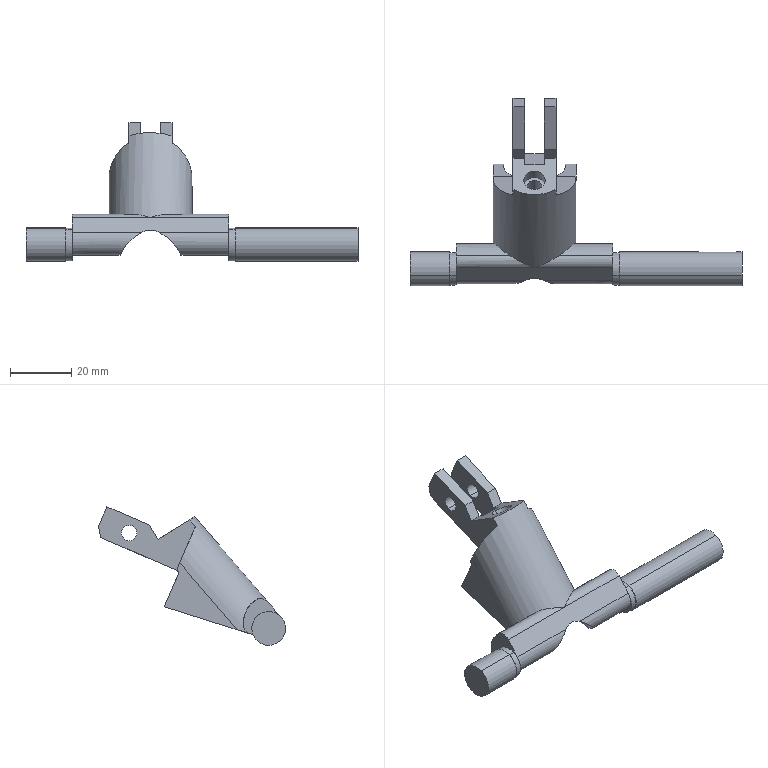Part | SolidWorks | features BaseBody 1 | 1 solid | 73 faces | box 108 x 60.896 x 45.086 mm | volume 20880 mm3 | plane 41 | cylinder 32 | commonest cylinder face diameters 5 x6 6 x6 10.6 x4 11 x4 7 x2 9 x2